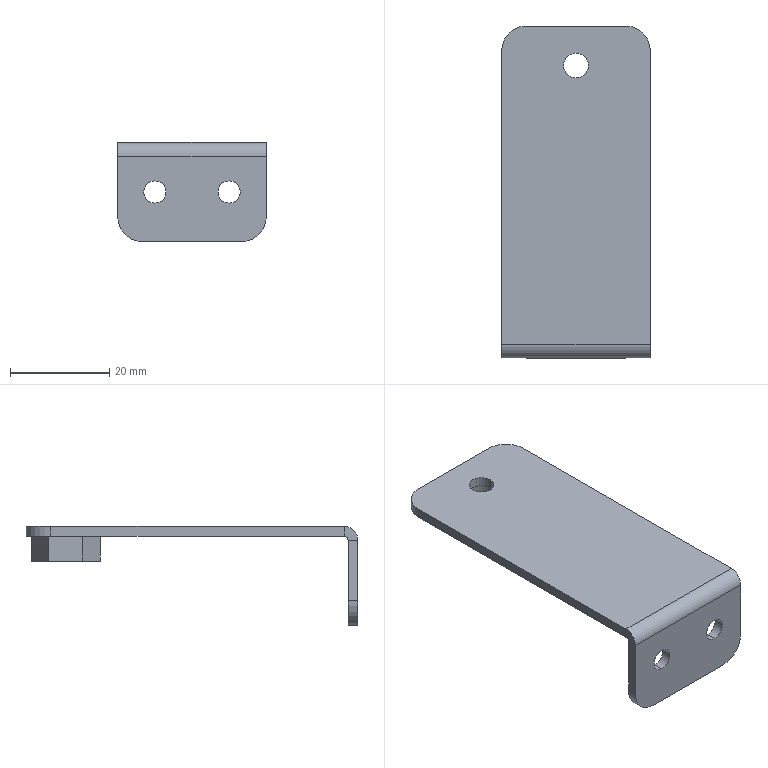Part | STEP file | 1 solid | 34 faces | box 30 x 67 x 20 mm | volume 5371 mm3 | plane 20 | cylinder 14 | commonest cylinder face diameters 4.5 x4 10 x4 5 x2 6.415 x2 1.473 x1 5.473 x1